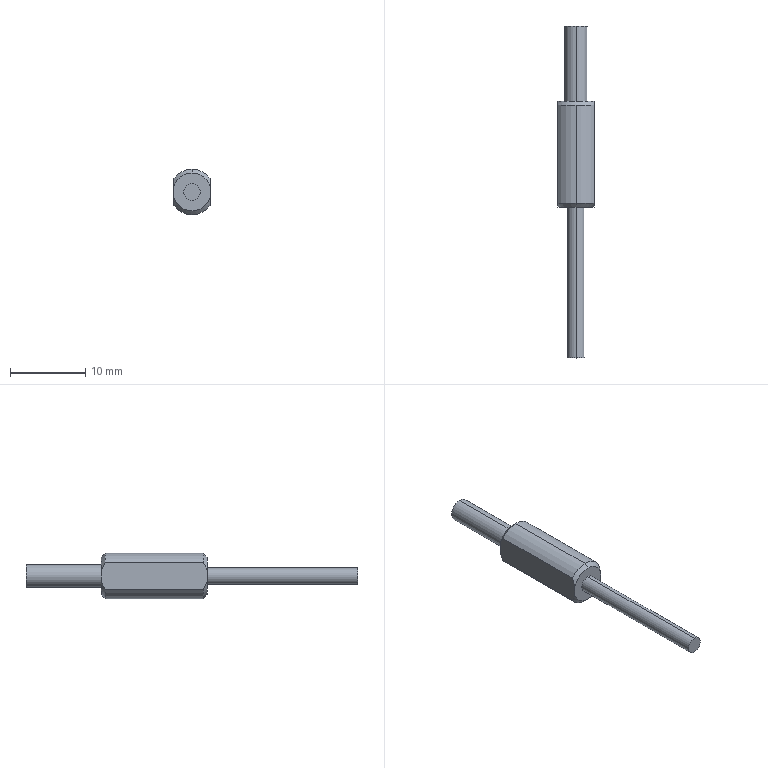Part | SolidWorks | features ICE 3, Chamfer 1, Extrusion 1, MirrorPattern 1 | 1 solid | 19 faces | box 4.8 x 44 x 6 mm | volume 498.476 mm3 | cylinder 7 | cone 6 | plane 6 | commonest cylinder face diameters 6 x3 2.2 x2 3 x2
STEP:
#1=CARTESIAN_POINT('',(0.,-34.,-1.1));
#2=VERTEX_POINT('',#1);
#3=CARTESIAN_POINT('',(0.,-34.,1.1));
#4=VERTEX_POINT('',#3);
#5=CARTESIAN_POINT('',(0.,-34.,0.));
#6=DIRECTION('',(0.,-1.,0.));
#7=DIRECTION('',(0.,0.,-1.));
#8=AXIS2_PLACEMENT_3D('',#5,#6,#7);
#9=CIRCLE('',#8,1.1);
#10=EDGE_CURVE('',#2,#4,#9,.T.);
#11=ORIENTED_EDGE('',*,*,#10,.F.);
#12=CARTESIAN_POINT('',(0.,-14.,-1.1));
#13=VERTEX_POINT('',#12);
#14=CARTESIAN_POINT('',(0.,-34.,-1.1));
#15=DIRECTION('',(0.,1.,0.));
#16=VECTOR('',#15,1000.);
#17=LINE('',#14,#16);
#18=EDGE_CURVE('',#2,#13,#17,.T.);
#19=ORIENTED_EDGE('',*,*,#18,.T.);
#20=CARTESIAN_POINT('',(0.,-14.,1.1));
#21=VERTEX_POINT('',#20);
#22=CARTESIAN_POINT('',(0.,-14.,0.));
#23=DIRECTION('',(0.,-1.,0.));
#24=DIRECTION('',(0.,0.,-1.));
#25=AXIS2_PLACEMENT_3D('',#22,#23,#24);
#26=CIRCLE('',#25,1.1);
#27=EDGE_CURVE('',#13,#21,#26,.T.);
#28=ORIENTED_EDGE('',*,*,#27,.T.);
#29=CARTESIAN_POINT('',(0.,-34.,1.1));
#30=DIRECTION('',(0.,1.,0.));
#31=VECTOR('',#30,1000.);
#32=LINE('',#29,#31);
#33=EDGE_CURVE('',#4,#21,#32,.T.);
#34=ORIENTED_EDGE('',*,*,#33,.F.);
#35=EDGE_LOOP('',(#11,#19,#28,#34));
#36=FACE_OUTER_BOUND('',#35,.T.);
#37=CARTESIAN_POINT('',(0.,-34.,0.));
#38=DIRECTION('',(0.,1.,0.));
#39=DIRECTION('',(0.,0.,1.));
#40=AXIS2_PLACEMENT_3D('',#37,#38,#39);
#41=CYLINDRICAL_SURFACE('',#40,1.1);
#42=ADVANCED_FACE('',(#36),#41,.T.);
#43=CARTESIAN_POINT('',(0.,10.,1.5));
#44=VERTEX_POINT('',#43);
#45=CARTESIAN_POINT('',(0.,10.,-1.5));
#46=VERTEX_POINT('',#45);
#47=CARTESIAN_POINT('',(0.,10.,0.));
#48=DIRECTION('',(0.,1.,0.));
#49=DIRECTION('',(0.,0.,1.));
#50=AXIS2_PLACEMENT_3D('',#47,#48,#49);
#51=CIRCLE('',#50,1.5);
#52=EDGE_CURVE('',#44,#46,#51,.T.);
#53=ORIENTED_EDGE('',*,*,#52,.F.);
#54=CARTESIAN_POINT('',(0.,0.,1.5));
#55=VERTEX_POINT('',#54);
#56=CARTESIAN_POINT('',(0.,10.,1.5));
#57=DIRECTION('',(0.,-1.,0.));
#58=VECTOR('',#57,1000.);
#59=LINE('',#56,#58);
#60=EDGE_CURVE('',#44,#55,#59,.T.);
#61=ORIENTED_EDGE('',*,*,#60,.T.);
#62=CARTESIAN_POINT('',(0.,0.,-1.5));
#63=VERTEX_POINT('',#62);
#64=CARTESIAN_POINT('',(0.,0.,0.));
#65=DIRECTION('',(0.,-1.,0.));
#66=DIRECTION('',(0.,0.,-1.));
#67=AXIS2_PLACEMENT_3D('',#64,#65,#66);
#68=CIRCLE('',#67,1.5);
#69=EDGE_CURVE('',#63,#55,#68,.T.);
#70=ORIENTED_EDGE('',*,*,#69,.F.);
#71=CARTESIAN_POINT('',(0.,10.,-1.5));
#72=DIRECTION('',(0.,-1.,0.));
#73=VECTOR('',#72,1000.);
#74=LINE('',#71,#73);
#75=EDGE_CURVE('',#46,#63,#74,.T.);
#76=ORIENTED_EDGE('',*,*,#75,.F.);
#77=EDGE_LOOP('',(#53,#61,#70,#76));
#78=FACE_OUTER_BOUND('',#77,.T.);
#79=CARTESIAN_POINT('',(0.,10.,0.));
#80=DIRECTION('',(0.,-1.,0.));
#81=DIRECTION('',(0.,0.,-1.));
#82=AXIS2_PLACEMENT_3D('',#79,#80,#81);
#83=CYLINDRICAL_SURFACE('',#82,1.5);
#84=ADVANCED_FACE('',(#78),#83,.T.);
#85=CARTESIAN_POINT('',(0.,0.,-2.5));
#86=VERTEX_POINT('',#85);
#87=CARTESIAN_POINT('',(-2.4,0.,-0.7));
#88=VERTEX_POINT('',#87);
#89=CARTESIAN_POINT('',(0.,0.,0.));
#90=DIRECTION('',(0.,1.,0.));
#91=DIRECTION('',(0.,0.,-1.));
#92=AXIS2_PLACEMENT_3D('',#89,#90,#91);
#93=CIRCLE('',#92,2.5);
#94=EDGE_CURVE('',#86,#88,#93,.T.);
#95=ORIENTED_EDGE('',*,*,#94,.F.);
#96=CARTESIAN_POINT('',(0.,-0.5,-3.));
#97=VERTEX_POINT('',#96);
#98=CARTESIAN_POINT('',(0.,-0.5,-3.));
#99=DIRECTION('',(0.,-0.7071,-0.7071));
#100=VECTOR('',#99,1000.);
#101=LINE('',#98,#100);
#102=EDGE_CURVE('',#86,#97,#101,.T.);
#103=ORIENTED_EDGE('',*,*,#102,.T.);
#104=CARTESIAN_POINT('',(-2.4,-0.5,-1.8));
#105=VERTEX_POINT('',#104);
#106=CARTESIAN_POINT('',(0.,-0.5,0.));
#107=DIRECTION('',(0.,-1.,0.));
#108=DIRECTION('',(0.,0.,-1.));
#109=AXIS2_PLACEMENT_3D('',#106,#107,#108);
#110=CIRCLE('',#109,3.);
#111=EDGE_CURVE('',#105,#97,#110,.T.);
#112=ORIENTED_EDGE('',*,*,#111,.F.);
#113=CARTESIAN_POINT('',(-2.4,-0.5,-1.8));
#114=CARTESIAN_POINT('',(-2.4,-0.3959,-1.627));
#115=CARTESIAN_POINT('',(-2.4,-0.2991,-1.45));
#116=CARTESIAN_POINT('',(-2.4,-0.1286,-1.084));
#117=CARTESIAN_POINT('',(-2.4,-0.0544,-0.8943));
#118=CARTESIAN_POINT('',(-2.4,0.,-0.7));
#119=B_SPLINE_CURVE_WITH_KNOTS('',3,(#113,#114,#115,#116,#117,#118),.UNSPECIFIED.,.F.,.F.,(4,2,4),(0.005672,0.006278,0.006883),.UNSPECIFIED.);
#120=EDGE_CURVE('',#105,#88,#119,.T.);
#121=ORIENTED_EDGE('',*,*,#120,.T.);
#122=EDGE_LOOP('',(#95,#103,#112,#121));
#123=FACE_OUTER_BOUND('',#122,.T.);
#124=CARTESIAN_POINT('',(0.,-0.5,0.));
#125=DIRECTION('',(0.,-1.,0.));
#126=DIRECTION('',(0.,0.,-1.));
#127=AXIS2_PLACEMENT_3D('',#124,#125,#126);
#128=CONICAL_SURFACE('',#127,3.,0.7854);
#129=ADVANCED_FACE('',(#123),#128,.T.);
#130=CARTESIAN_POINT('',(0.,-14.,2.5));
#131=VERTEX_POINT('',#130);
#132=CARTESIAN_POINT('',(-2.4,-14.,0.7));
#133=VERTEX_POINT('',#132);
#134=CARTESIAN_POINT('',(0.,-14.,0.));
#135=DIRECTION('',(0.,-1.,0.));
#136=DIRECTION('',(0.,0.,-1.));
#137=AXIS2_PLACEMENT_3D('',#134,#135,#136);
#138=CIRCLE('',#137,2.5);
#139=EDGE_CURVE('',#131,#133,#138,.T.);
#140=ORIENTED_EDGE('',*,*,#139,.F.);
#141=CARTESIAN_POINT('',(0.,-13.5,3.));
#142=VERTEX_POINT('',#141);
#143=CARTESIAN_POINT('',(0.,-14.,2.5));
#144=DIRECTION('',(0.,0.7071,0.7071));
#145=VECTOR('',#144,1000.);
#146=LINE('',#143,#145);
#147=EDGE_CURVE('',#131,#142,#146,.T.);
#148=ORIENTED_EDGE('',*,*,#147,.T.);
#149=CARTESIAN_POINT('',(-2.4,-13.5,1.8));
#150=VERTEX_POINT('',#149);
#151=CARTESIAN_POINT('',(0.,-13.5,0.));
#152=DIRECTION('',(0.,1.,0.));
#153=DIRECTION('',(0.,0.,-1.));
#154=AXIS2_PLACEMENT_3D('',#151,#152,#153);
#155=CIRCLE('',#154,3.);
#156=EDGE_CURVE('',#150,#142,#155,.T.);
#157=ORIENTED_EDGE('',*,*,#156,.F.);
#158=CARTESIAN_POINT('',(-2.4,-13.5,1.8));
#159=CARTESIAN_POINT('',(-2.4,-13.604,1.627));
#160=CARTESIAN_POINT('',(-2.4,-13.701,1.45));
#161=CARTESIAN_POINT('',(-2.4,-13.871,1.084));
#162=CARTESIAN_POINT('',(-2.4,-13.946,0.8943));
#163=CARTESIAN_POINT('',(-2.4,-14.,0.7));
#164=B_SPLINE_CURVE_WITH_KNOTS('',3,(#158,#159,#160,#161,#162,#163),.UNSPECIFIED.,.F.,.F.,(4,2,4),(0.005672,0.006278,0.006883),.UNSPECIFIED.);
#165=EDGE_CURVE('',#150,#133,#164,.T.);
#166=ORIENTED_EDGE('',*,*,#165,.T.);
#167=EDGE_LOOP('',(#140,#148,#157,#166));
#168=FACE_OUTER_BOUND('',#167,.T.);
#169=CARTESIAN_POINT('',(0.,-14.,0.));
#170=DIRECTION('',(0.,1.,0.));
#171=DIRECTION('',(0.,0.,1.));
#172=AXIS2_PLACEMENT_3D('',#169,#170,#171);
#173=CONICAL_SURFACE('',#172,2.5,0.7854);
#174=ADVANCED_FACE('',(#168),#173,.T.);
#175=ORIENTED_EDGE('',*,*,#156,.T.);
#176=CARTESIAN_POINT('',(0.,-0.5,3.));
#177=VERTEX_POINT('',#176);
#178=CARTESIAN_POINT('',(0.,-14.,3.));
#179=DIRECTION('',(0.,1.,0.));
#180=VECTOR('',#179,1000.);
#181=LINE('',#178,#180);
#182=EDGE_CURVE('',#142,#177,#181,.T.);
#183=ORIENTED_EDGE('',*,*,#182,.T.);
#184=CARTESIAN_POINT('',(-2.4,-0.5,1.8));
#185=VERTEX_POINT('',#184);
#186=CARTESIAN_POINT('',(0.,-0.5,0.));
#187=DIRECTION('',(0.,-1.,0.));
#188=DIRECTION('',(0.,0.,-1.));
#189=AXIS2_PLACEMENT_3D('',#186,#187,#188);
#190=CIRCLE('',#189,3.);
#191=EDGE_CURVE('',#177,#185,#190,.T.);
#192=ORIENTED_EDGE('',*,*,#191,.T.);
#193=CARTESIAN_POINT('',(-2.4,-14.,1.8));
#194=DIRECTION('',(0.,1.,0.));
#195=VECTOR('',#194,1000.);
#196=LINE('',#193,#195);
#197=EDGE_CURVE('',#150,#185,#196,.T.);
#198=ORIENTED_EDGE('',*,*,#197,.F.);
#199=EDGE_LOOP('',(#175,#183,#192,#198));
#200=FACE_OUTER_BOUND('',#199,.T.);
#201=CARTESIAN_POINT('',(0.,-14.,0.));
#202=DIRECTION('',(0.,1.,0.));
#203=DIRECTION('',(0.,0.,1.));
#204=AXIS2_PLACEMENT_3D('',#201,#202,#203);
#205=CYLINDRICAL_SURFACE('',#204,3.);
#206=ADVANCED_FACE('',(#200),#205,.T.);
#207=CARTESIAN_POINT('',(0.,-14.,0.));
#208=DIRECTION('',(0.,-1.,0.));
#209=DIRECTION('',(0.,0.,-1.));
#210=AXIS2_PLACEMENT_3D('',#207,#208,#209);
#211=CIRCLE('',#210,1.1);
#212=EDGE_CURVE('',#21,#13,#211,.T.);
#213=ORIENTED_EDGE('',*,*,#212,.F.);
#214=ORIENTED_EDGE('',*,*,#27,.F.);
#215=EDGE_LOOP('',(#213,#214));
#216=FACE_BOUND('',#215,.T.);
#217=CARTESIAN_POINT('',(2.4,-14.,0.7));
#218=VERTEX_POINT('',#217);
#219=CARTESIAN_POINT('',(0.,-14.,0.));
#220=DIRECTION('',(0.,-1.,0.));
#221=DIRECTION('',(0.,0.,-1.));
#222=AXIS2_PLACEMENT_3D('',#219,#220,#221);
#223=CIRCLE('',#222,2.5);
#224=EDGE_CURVE('',#218,#131,#223,.T.);
#225=ORIENTED_EDGE('',*,*,#224,.T.);
#226=ORIENTED_EDGE('',*,*,#139,.T.);
#227=CARTESIAN_POINT('',(-2.4,-14.,-0.7));
#228=VERTEX_POINT('',#227);
#229=CARTESIAN_POINT('',(-2.4,-14.,0.));
#230=DIRECTION('',(0.,0.,-1.));
#231=VECTOR('',#230,1000.);
#232=LINE('',#229,#231);
#233=EDGE_CURVE('',#133,#228,#232,.T.);
#234=ORIENTED_EDGE('',*,*,#233,.T.);
#235=CARTESIAN_POINT('',(2.4,-14.,-0.7));
#236=VERTEX_POINT('',#235);
#237=CARTESIAN_POINT('',(0.,-14.,0.));
#238=DIRECTION('',(0.,-1.,0.));
#239=DIRECTION('',(0.,0.,-1.));
#240=AXIS2_PLACEMENT_3D('',#237,#238,#239);
#241=CIRCLE('',#240,2.5);
#242=EDGE_CURVE('',#228,#236,#241,.T.);
#243=ORIENTED_EDGE('',*,*,#242,.T.);
#244=CARTESIAN_POINT('',(2.4,-14.,0.));
#245=DIRECTION('',(0.,0.,-1.));
#246=VECTOR('',#245,1000.);
#247=LINE('',#244,#246);
#248=EDGE_CURVE('',#218,#236,#247,.T.);
#249=ORIENTED_EDGE('',*,*,#248,.F.);
#250=EDGE_LOOP('',(#225,#226,#234,#243,#249));
#251=FACE_OUTER_BOUND('',#250,.T.);
#252=CARTESIAN_POINT('',(0.,-14.,0.));
#253=DIRECTION('',(0.,-1.,0.));
#254=DIRECTION('',(0.,0.,-1.));
#255=AXIS2_PLACEMENT_3D('',#252,#253,#254);
#256=PLANE('',#255);
#257=ADVANCED_FACE('',(#216,#251),#256,.T.);
#258=ORIENTED_EDGE('',*,*,#69,.T.);
#259=CARTESIAN_POINT('',(0.,0.,0.));
#260=DIRECTION('',(0.,-1.,0.));
#261=DIRECTION('',(0.,0.,-1.));
#262=AXIS2_PLACEMENT_3D('',#259,#260,#261);
#263=CIRCLE('',#262,1.5);
#264=EDGE_CURVE('',#55,#63,#263,.T.);
#265=ORIENTED_EDGE('',*,*,#264,.T.);
#266=EDGE_LOOP('',(#258,#265));
#267=FACE_BOUND('',#266,.T.);
#268=CARTESIAN_POINT('',(-2.4,0.,0.7));
#269=VERTEX_POINT('',#268);
#270=CARTESIAN_POINT('',(-2.4,0.,0.));
#271=DIRECTION('',(0.,0.,-1.));
#272=VECTOR('',#271,1000.);
#273=LINE('',#270,#272);
#274=EDGE_CURVE('',#269,#88,#273,.T.);
#275=ORIENTED_EDGE('',*,*,#274,.F.);
#276=CARTESIAN_POINT('',(2.4,0.,0.7));
#277=VERTEX_POINT('',#276);
#278=CARTESIAN_POINT('',(0.,0.,0.));
#279=DIRECTION('',(0.,1.,0.));
#280=DIRECTION('',(0.,0.,-1.));
#281=AXIS2_PLACEMENT_3D('',#278,#279,#280);
#282=CIRCLE('',#281,2.5);
#283=EDGE_CURVE('',#269,#277,#282,.T.);
#284=ORIENTED_EDGE('',*,*,#283,.T.);
#285=CARTESIAN_POINT('',(2.4,0.,-0.7));
#286=VERTEX_POINT('',#285);
#287=CARTESIAN_POINT('',(2.4,0.,0.));
#288=DIRECTION('',(0.,0.,-1.));
#289=VECTOR('',#288,1000.);
#290=LINE('',#287,#289);
#291=EDGE_CURVE('',#277,#286,#290,.T.);
#292=ORIENTED_EDGE('',*,*,#291,.T.);
#293=CARTESIAN_POINT('',(0.,0.,0.));
#294=DIRECTION('',(0.,1.,0.));
#295=DIRECTION('',(0.,0.,-1.));
#296=AXIS2_PLACEMENT_3D('',#293,#294,#295);
#297=CIRCLE('',#296,2.5);
#298=EDGE_CURVE('',#286,#86,#297,.T.);
#299=ORIENTED_EDGE('',*,*,#298,.T.);
#300=ORIENTED_EDGE('',*,*,#94,.T.);
#301=EDGE_LOOP('',(#275,#284,#292,#299,#300));
#302=FACE_OUTER_BOUND('',#301,.T.);
#303=CARTESIAN_POINT('',(0.,0.,0.));
#304=DIRECTION('',(0.,-1.,0.));
#305=DIRECTION('',(0.,0.,-1.));
#306=AXIS2_PLACEMENT_3D('',#303,#304,#305);
#307=PLANE('',#306);
#308=ADVANCED_FACE('',(#267,#302),#307,.F.);
#309=ORIENTED_EDGE('',*,*,#182,.F.);
#310=CARTESIAN_POINT('',(2.4,-13.5,1.8));
#311=VERTEX_POINT('',#310);
#312=CARTESIAN_POINT('',(0.,-13.5,0.));
#313=DIRECTION('',(0.,1.,0.));
#314=DIRECTION('',(0.,0.,-1.));
#315=AXIS2_PLACEMENT_3D('',#312,#313,#314);
#316=CIRCLE('',#315,3.);
#317=EDGE_CURVE('',#142,#311,#316,.T.);
#318=ORIENTED_EDGE('',*,*,#317,.T.);
#319=CARTESIAN_POINT('',(2.4,-0.5,1.8));
#320=VERTEX_POINT('',#319);
#321=CARTESIAN_POINT('',(2.4,-14.,1.8));
#322=DIRECTION('',(0.,1.,0.));
#323=VECTOR('',#322,1000.);
#324=LINE('',#321,#323);
#325=EDGE_CURVE('',#311,#320,#324,.T.);
#326=ORIENTED_EDGE('',*,*,#325,.T.);
#327=CARTESIAN_POINT('',(0.,-0.5,0.));
#328=DIRECTION('',(0.,-1.,0.));
#329=DIRECTION('',(0.,0.,-1.));
#330=AXIS2_PLACEMENT_3D('',#327,#328,#329);
#331=CIRCLE('',#330,3.);
#332=EDGE_CURVE('',#320,#177,#331,.T.);
#333=ORIENTED_EDGE('',*,*,#332,.T.);
#334=EDGE_LOOP('',(#309,#318,#326,#333));
#335=FACE_OUTER_BOUND('',#334,.T.);
#336=CARTESIAN_POINT('',(0.,-14.,0.));
#337=DIRECTION('',(0.,1.,0.));
#338=DIRECTION('',(0.,0.,1.));
#339=AXIS2_PLACEMENT_3D('',#336,#337,#338);
#340=CYLINDRICAL_SURFACE('',#339,3.);
#341=ADVANCED_FACE('',(#335),#340,.T.);
#342=CARTESIAN_POINT('',(-2.4,-13.5,-1.8));
#343=VERTEX_POINT('',#342);
#344=CARTESIAN_POINT('',(-2.4,-14.,-1.8));
#345=DIRECTION('',(0.,-1.,0.));
#346=VECTOR('',#345,1000.);
#347=LINE('',#344,#346);
#348=EDGE_CURVE('',#105,#343,#347,.T.);
#349=ORIENTED_EDGE('',*,*,#348,.F.);
#350=ORIENTED_EDGE('',*,*,#111,.T.);
#351=CARTESIAN_POINT('',(2.4,-0.5,-1.8));
#352=VERTEX_POINT('',#351);
#353=CARTESIAN_POINT('',(0.,-0.5,0.));
#354=DIRECTION('',(0.,-1.,0.));
#355=DIRECTION('',(0.,0.,-1.));
#356=AXIS2_PLACEMENT_3D('',#353,#354,#355);
#357=CIRCLE('',#356,3.);
#358=EDGE_CURVE('',#97,#352,#357,.T.);
#359=ORIENTED_EDGE('',*,*,#358,.T.);
#360=CARTESIAN_POINT('',(2.4,-13.5,-1.8));
#361=VERTEX_POINT('',#360);
#362=CARTESIAN_POINT('',(2.4,-14.,-1.8));
#363=DIRECTION('',(0.,-1.,0.));
#364=VECTOR('',#363,1000.);
#365=LINE('',#362,#364);
#366=EDGE_CURVE('',#352,#361,#365,.T.);
#367=ORIENTED_EDGE('',*,*,#366,.T.);
#368=CARTESIAN_POINT('',(0.,-13.5,0.));
#369=DIRECTION('',(0.,1.,0.));
#370=DIRECTION('',(0.,0.,-1.));
#371=AXIS2_PLACEMENT_3D('',#368,#369,#370);
#372=CIRCLE('',#371,3.);
#373=EDGE_CURVE('',#361,#343,#372,.T.);
#374=ORIENTED_EDGE('',*,*,#373,.T.);
#375=EDGE_LOOP('',(#349,#350,#359,#367,#374));
#376=FACE_OUTER_BOUND('',#375,.T.);
#377=CARTESIAN_POINT('',(0.,-14.,0.));
#378=DIRECTION('',(0.,1.,0.));
#379=DIRECTION('',(0.,0.,1.));
#380=AXIS2_PLACEMENT_3D('',#377,#378,#379);
#381=CYLINDRICAL_SURFACE('',#380,3.);
#382=ADVANCED_FACE('',(#376),#381,.T.);
#383=ORIENTED_EDGE('',*,*,#147,.F.);
#384=ORIENTED_EDGE('',*,*,#224,.F.);
#385=CARTESIAN_POINT('',(2.4,-13.5,1.8));
#386=CARTESIAN_POINT('',(2.4,-13.604,1.627));
#387=CARTESIAN_POINT('',(2.4,-13.701,1.45));
#388=CARTESIAN_POINT('',(2.4,-13.871,1.084));
#389=CARTESIAN_POINT('',(2.4,-13.946,0.8943));
#390=CARTESIAN_POINT('',(2.4,-14.,0.7));
#391=B_SPLINE_CURVE_WITH_KNOTS('',3,(#385,#386,#387,#388,#389,#390),.UNSPECIFIED.,.F.,.F.,(4,2,4),(0.005672,0.006278,0.006883),.UNSPECIFIED.);
#392=EDGE_CURVE('',#311,#218,#391,.T.);
#393=ORIENTED_EDGE('',*,*,#392,.F.);
#394=ORIENTED_EDGE('',*,*,#317,.F.);
#395=EDGE_LOOP('',(#383,#384,#393,#394));
#396=FACE_OUTER_BOUND('',#395,.T.);
#397=CARTESIAN_POINT('',(0.,-14.,0.));
#398=DIRECTION('',(0.,1.,0.));
#399=DIRECTION('',(0.,0.,1.));
#400=AXIS2_PLACEMENT_3D('',#397,#398,#399);
#401=CONICAL_SURFACE('',#400,2.5,0.7854);
#402=ADVANCED_FACE('',(#396),#401,.T.);
#403=ORIENTED_EDGE('',*,*,#242,.F.);
#404=CARTESIAN_POINT('',(-2.4,-14.,-0.7));
#405=CARTESIAN_POINT('',(-2.4,-13.945,-0.8954));
#406=CARTESIAN_POINT('',(-2.4,-13.87,-1.086));
#407=CARTESIAN_POINT('',(-2.4,-13.7,-1.452));
#408=CARTESIAN_POINT('',(-2.4,-13.603,-1.628));
#409=CARTESIAN_POINT('',(-2.4,-13.5,-1.8));
#410=B_SPLINE_CURVE_WITH_KNOTS('',3,(#404,#405,#406,#407,#408,#409),.UNSPECIFIED.,.F.,.F.,(4,2,4),(0.008304,0.008913,0.009522),.UNSPECIFIED.);
#411=EDGE_CURVE('',#228,#343,#410,.T.);
#412=ORIENTED_EDGE('',*,*,#411,.T.);
#413=ORIENTED_EDGE('',*,*,#373,.F.);
#414=CARTESIAN_POINT('',(2.4,-14.,-0.7));
#415=CARTESIAN_POINT('',(2.4,-13.945,-0.8954));
#416=CARTESIAN_POINT('',(2.4,-13.87,-1.086));
#417=CARTESIAN_POINT('',(2.4,-13.7,-1.452));
#418=CARTESIAN_POINT('',(2.4,-13.603,-1.628));
#419=CARTESIAN_POINT('',(2.4,-13.5,-1.8));
#420=B_SPLINE_CURVE_WITH_KNOTS('',3,(#414,#415,#416,#417,#418,#419),.UNSPECIFIED.,.F.,.F.,(4,2,4),(0.008304,0.008913,0.009522),.UNSPECIFIED.);
#421=EDGE_CURVE('',#236,#361,#420,.T.);
#422=ORIENTED_EDGE('',*,*,#421,.F.);
#423=EDGE_LOOP('',(#403,#412,#413,#422));
#424=FACE_OUTER_BOUND('',#423,.T.);
#425=CARTESIAN_POINT('',(0.,-14.,0.));
#426=DIRECTION('',(0.,1.,0.));
#427=DIRECTION('',(0.,0.,1.));
#428=AXIS2_PLACEMENT_3D('',#425,#426,#427);
#429=CONICAL_SURFACE('',#428,2.5,0.7854);
#430=ADVANCED_FACE('',(#424),#429,.T.);
#431=ORIENTED_EDGE('',*,*,#102,.F.);
#432=ORIENTED_EDGE('',*,*,#298,.F.);
#433=CARTESIAN_POINT('',(2.4,-0.5,-1.8));
#434=CARTESIAN_POINT('',(2.4,-0.3959,-1.627));
#435=CARTESIAN_POINT('',(2.4,-0.2991,-1.45));
#436=CARTESIAN_POINT('',(2.4,-0.1286,-1.084));
#437=CARTESIAN_POINT('',(2.4,-0.0544,-0.8943));
#438=CARTESIAN_POINT('',(2.4,0.,-0.7));
#439=B_SPLINE_CURVE_WITH_KNOTS('',3,(#433,#434,#435,#436,#437,#438),.UNSPECIFIED.,.F.,.F.,(4,2,4),(0.005672,0.006278,0.006883),.UNSPECIFIED.);
#440=EDGE_CURVE('',#352,#286,#439,.T.);
#441=ORIENTED_EDGE('',*,*,#440,.F.);
#442=ORIENTED_EDGE('',*,*,#358,.F.);
#443=EDGE_LOOP('',(#431,#432,#441,#442));
#444=FACE_OUTER_BOUND('',#443,.T.);
#445=CARTESIAN_POINT('',(0.,-0.5,0.));
#446=DIRECTION('',(0.,-1.,0.));
#447=DIRECTION('',(0.,0.,-1.));
#448=AXIS2_PLACEMENT_3D('',#445,#446,#447);
#449=CONICAL_SURFACE('',#448,3.,0.7854);
#450=ADVANCED_FACE('',(#444),#449,.T.);
#451=ORIENTED_EDGE('',*,*,#283,.F.);
#452=CARTESIAN_POINT('',(-2.4,0.,0.7));
#453=CARTESIAN_POINT('',(-2.4,-0.05471,0.8954));
#454=CARTESIAN_POINT('',(-2.4,-0.1295,1.086));
#455=CARTESIAN_POINT('',(-2.4,-0.3002,1.452));
#456=CARTESIAN_POINT('',(-2.4,-0.3966,1.628));
#457=CARTESIAN_POINT('',(-2.4,-0.5,1.8));
#458=B_SPLINE_CURVE_WITH_KNOTS('',3,(#452,#453,#454,#455,#456,#457),.UNSPECIFIED.,.F.,.F.,(4,2,4),(0.008304,0.008913,0.009522),.UNSPECIFIED.);
#459=EDGE_CURVE('',#269,#185,#458,.T.);
#460=ORIENTED_EDGE('',*,*,#459,.T.);
#461=ORIENTED_EDGE('',*,*,#191,.F.);
#462=ORIENTED_EDGE('',*,*,#332,.F.);
#463=CARTESIAN_POINT('',(2.4,0.,0.7));
#464=CARTESIAN_POINT('',(2.4,-0.05471,0.8954));
#465=CARTESIAN_POINT('',(2.4,-0.1295,1.086));
#466=CARTESIAN_POINT('',(2.4,-0.3002,1.452));
#467=CARTESIAN_POINT('',(2.4,-0.3966,1.628));
#468=CARTESIAN_POINT('',(2.4,-0.5,1.8));
#469=B_SPLINE_CURVE_WITH_KNOTS('',3,(#463,#464,#465,#466,#467,#468),.UNSPECIFIED.,.F.,.F.,(4,2,4),(0.008304,0.008913,0.009522),.UNSPECIFIED.);
#470=EDGE_CURVE('',#277,#320,#469,.T.);
#471=ORIENTED_EDGE('',*,*,#470,.F.);
#472=EDGE_LOOP('',(#451,#460,#461,#462,#471));
#473=FACE_OUTER_BOUND('',#472,.T.);
#474=CARTESIAN_POINT('',(0.,-0.5,0.));
#475=DIRECTION('',(0.,-1.,0.));
#476=DIRECTION('',(0.,0.,-1.));
#477=AXIS2_PLACEMENT_3D('',#474,#475,#476);
#478=CONICAL_SURFACE('',#477,3.,0.7854);
#479=ADVANCED_FACE('',(#473),#478,.T.);
#480=ORIENTED_EDGE('',*,*,#60,.F.);
#481=CARTESIAN_POINT('',(0.,10.,0.));
#482=DIRECTION('',(0.,1.,0.));
#483=DIRECTION('',(0.,0.,1.));
#484=AXIS2_PLACEMENT_3D('',#481,#482,#483);
#485=CIRCLE('',#484,1.5);
#486=EDGE_CURVE('',#46,#44,#485,.T.);
#487=ORIENTED_EDGE('',*,*,#486,.F.);
#488=ORIENTED_EDGE('',*,*,#75,.T.);
#489=ORIENTED_EDGE('',*,*,#264,.F.);
#490=EDGE_LOOP('',(#480,#487,#488,#489));
#491=FACE_OUTER_BOUND('',#490,.T.);
#492=CARTESIAN_POINT('',(0.,10.,0.));
#493=DIRECTION('',(0.,-1.,0.));
#494=DIRECTION('',(0.,0.,-1.));
#495=AXIS2_PLACEMENT_3D('',#492,#493,#494);
#496=CYLINDRICAL_SURFACE('',#495,1.5);
#497=ADVANCED_FACE('',(#491),#496,.T.);
#498=ORIENTED_EDGE('',*,*,#486,.T.);
#499=ORIENTED_EDGE('',*,*,#52,.T.);
#500=EDGE_LOOP('',(#498,#499));
#501=FACE_OUTER_BOUND('',#500,.T.);
#502=CARTESIAN_POINT('',(0.,10.,0.));
#503=DIRECTION('',(0.,1.,0.));
#504=DIRECTION('',(0.,0.,1.));
#505=AXIS2_PLACEMENT_3D('',#502,#503,#504);
#506=PLANE('',#505);
#507=ADVANCED_FACE('',(#501),#506,.T.);
#508=ORIENTED_EDGE('',*,*,#18,.F.);
#509=CARTESIAN_POINT('',(0.,-34.,0.));
#510=DIRECTION('',(0.,-1.,0.));
#511=DIRECTION('',(0.,0.,-1.));
#512=AXIS2_PLACEMENT_3D('',#509,#510,#511);
#513=CIRCLE('',#512,1.1);
#514=EDGE_CURVE('',#4,#2,#513,.T.);
#515=ORIENTED_EDGE('',*,*,#514,.F.);
#516=ORIENTED_EDGE('',*,*,#33,.T.);
#517=ORIENTED_EDGE('',*,*,#212,.T.);
#518=EDGE_LOOP('',(#508,#515,#516,#517));
#519=FACE_OUTER_BOUND('',#518,.T.);
#520=CARTESIAN_POINT('',(0.,-34.,0.));
#521=DIRECTION('',(0.,1.,0.));
#522=DIRECTION('',(0.,0.,1.));
#523=AXIS2_PLACEMENT_3D('',#520,#521,#522);
#524=CYLINDRICAL_SURFACE('',#523,1.1);
#525=ADVANCED_FACE('',(#519),#524,.T.);
#526=ORIENTED_EDGE('',*,*,#514,.T.);
#527=ORIENTED_EDGE('',*,*,#10,.T.);
#528=EDGE_LOOP('',(#526,#527));
#529=FACE_OUTER_BOUND('',#528,.T.);
#530=CARTESIAN_POINT('',(0.,-34.,0.));
#531=DIRECTION('',(0.,-1.,0.));
#532=DIRECTION('',(0.,0.,-1.));
#533=AXIS2_PLACEMENT_3D('',#530,#531,#532);
#534=PLANE('',#533);
#535=ADVANCED_FACE('',(#529),#534,.T.);
#536=ORIENTED_EDGE('',*,*,#421,.T.);
#537=ORIENTED_EDGE('',*,*,#366,.F.);
#538=ORIENTED_EDGE('',*,*,#440,.T.);
#539=ORIENTED_EDGE('',*,*,#291,.F.);
#540=ORIENTED_EDGE('',*,*,#470,.T.);
#541=ORIENTED_EDGE('',*,*,#325,.F.);
#542=ORIENTED_EDGE('',*,*,#392,.T.);
#543=ORIENTED_EDGE('',*,*,#248,.T.);
#544=EDGE_LOOP('',(#536,#537,#538,#539,#540,#541,#542,#543));
#545=FACE_OUTER_BOUND('',#544,.T.);
#546=CARTESIAN_POINT('',(2.4,-34.,-3.797));
#547=DIRECTION('',(-1.,0.,0.));
#548=DIRECTION('',(0.,0.,1.));
#549=AXIS2_PLACEMENT_3D('',#546,#547,#548);
#550=PLANE('',#549);
#551=ADVANCED_FACE('',(#545),#550,.F.);
#552=ORIENTED_EDGE('',*,*,#233,.F.);
#553=ORIENTED_EDGE('',*,*,#165,.F.);
#554=ORIENTED_EDGE('',*,*,#197,.T.);
#555=ORIENTED_EDGE('',*,*,#459,.F.);
#556=ORIENTED_EDGE('',*,*,#274,.T.);
#557=ORIENTED_EDGE('',*,*,#120,.F.);
#558=ORIENTED_EDGE('',*,*,#348,.T.);
#559=ORIENTED_EDGE('',*,*,#411,.F.);
#560=EDGE_LOOP('',(#552,#553,#554,#555,#556,#557,#558,#559));
#561=FACE_OUTER_BOUND('',#560,.T.);
#562=CARTESIAN_POINT('',(-2.4,-34.,-3.797));
#563=DIRECTION('',(-1.,0.,0.));
#564=DIRECTION('',(0.,0.,1.));
#565=AXIS2_PLACEMENT_3D('',#562,#563,#564);
#566=PLANE('',#565);
#567=ADVANCED_FACE('',(#561),#566,.T.);
#568=CLOSED_SHELL('',(#42,#84,#129,#174,#206,#257,#308,#341,#382,#402,#430,#450,#479,#497,#507,#525,#535,#551,#567));
#569=MANIFOLD_SOLID_BREP('',#568);
#570=CARTESIAN_POINT('',(0.,0.,0.));
#571=DIRECTION('',(0.,0.,1.));
#572=DIRECTION('',(1.,0.,0.));
#573=AXIS2_PLACEMENT_3D('',#570,#571,#572);
#574=(LENGTH_UNIT()NAMED_UNIT(*)SI_UNIT(.MILLI.,.METRE.));
#575=UNCERTAINTY_MEASURE_WITH_UNIT(LENGTH_MEASURE(0.00001),#574,'','');
#576=(NAMED_UNIT(*)PLANE_ANGLE_UNIT()SI_UNIT($,.RADIAN.));
#577=(NAMED_UNIT(*)SI_UNIT($,.STERADIAN.)SOLID_ANGLE_UNIT());
#578=(GEOMETRIC_REPRESENTATION_CONTEXT(3)GLOBAL_UNCERTAINTY_ASSIGNED_CONTEXT((#575))GLOBAL_UNIT_ASSIGNED_CONTEXT((#574,#576,#577))REPRESENTATION_CONTEXT('',''));
#579=ADVANCED_BREP_SHAPE_REPRESENTATION('',(#569,#573),#578);